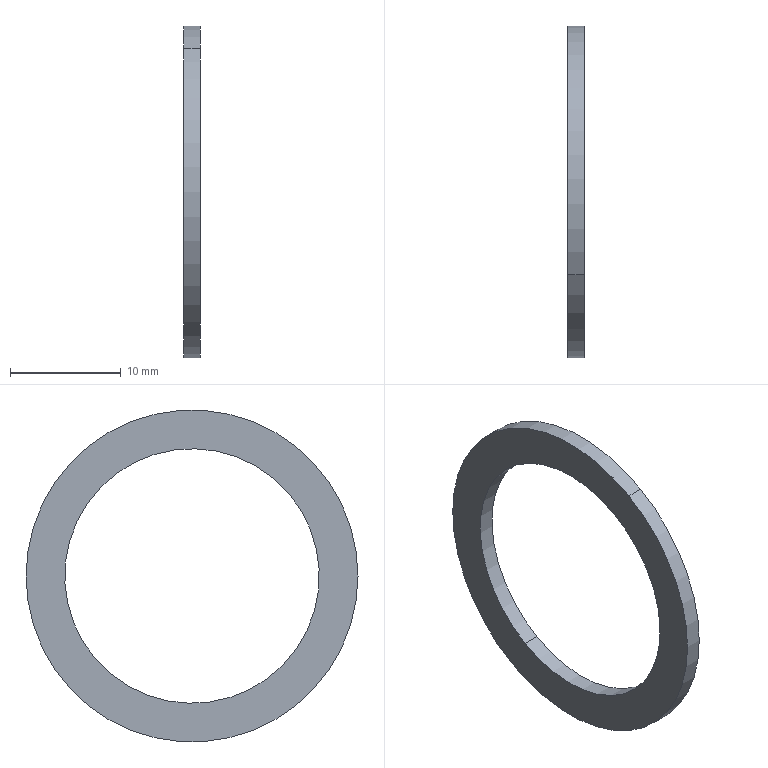Part | NX | features BREP 1 | 1 solid | 6 faces | box 1.5 x 30 x 30 mm | volume 437.074 mm3 | cylinder 4 | plane 2 | commonest cylinder face diameters 23 x2 30 x2
STEP:
#1=CARTESIAN_POINT('',(-605.855,39.831,-29.058));
#2=VERTEX_POINT('',#1);
#3=CARTESIAN_POINT('',(-605.855,51.331,-48.977));
#4=VERTEX_POINT('',#3);
#5=CARTESIAN_POINT('',(-605.855,45.581,-39.018));
#6=DIRECTION('',(-1.,0.,0.));
#7=DIRECTION('',(0.,0.5,-0.866));
#8=AXIS2_PLACEMENT_3D('',#5,#6,#7);
#9=CIRCLE('',#8,11.5);
#10=EDGE_CURVE('',#2,#4,#9,.T.);
#11=ORIENTED_EDGE('',*,*,#10,.T.);
#12=CARTESIAN_POINT('',(-604.355,51.331,-48.977));
#13=VERTEX_POINT('',#12);
#14=CARTESIAN_POINT('',(-605.855,51.331,-48.977));
#15=DIRECTION('',(-1.,0.,0.));
#16=VECTOR('',#15,1000.);
#17=LINE('',#14,#16);
#18=EDGE_CURVE('',#13,#4,#17,.T.);
#19=ORIENTED_EDGE('',*,*,#18,.F.);
#20=CARTESIAN_POINT('',(-604.355,39.831,-29.058));
#21=VERTEX_POINT('',#20);
#22=CARTESIAN_POINT('',(-604.355,45.581,-39.018));
#23=DIRECTION('',(-1.,0.,0.));
#24=DIRECTION('',(0.,0.5,-0.866));
#25=AXIS2_PLACEMENT_3D('',#22,#23,#24);
#26=CIRCLE('',#25,11.5);
#27=EDGE_CURVE('',#21,#13,#26,.T.);
#28=ORIENTED_EDGE('',*,*,#27,.F.);
#29=CARTESIAN_POINT('',(-605.855,39.831,-29.058));
#30=DIRECTION('',(-1.,0.,0.));
#31=VECTOR('',#30,1000.);
#32=LINE('',#29,#31);
#33=EDGE_CURVE('',#21,#2,#32,.T.);
#34=ORIENTED_EDGE('',*,*,#33,.T.);
#35=EDGE_LOOP('',(#11,#19,#28,#34));
#36=FACE_BOUND('',#35,.T.);
#37=CARTESIAN_POINT('',(-605.855,45.581,-39.018));
#38=DIRECTION('',(1.,0.,0.));
#39=DIRECTION('',(0.,-0.5,0.866));
#40=AXIS2_PLACEMENT_3D('',#37,#38,#39);
#41=CYLINDRICAL_SURFACE('',#40,11.5);
#42=ADVANCED_FACE('',(#36),#41,.F.);
#43=CARTESIAN_POINT('',(-605.855,53.081,-52.008));
#44=VERTEX_POINT('',#43);
#45=CARTESIAN_POINT('',(-605.855,38.081,-26.027));
#46=VERTEX_POINT('',#45);
#47=CARTESIAN_POINT('',(-605.855,45.581,-39.018));
#48=DIRECTION('',(-1.,0.,0.));
#49=DIRECTION('',(0.,0.5,-0.866));
#50=AXIS2_PLACEMENT_3D('',#47,#48,#49);
#51=CIRCLE('',#50,15.);
#52=EDGE_CURVE('',#44,#46,#51,.T.);
#53=ORIENTED_EDGE('',*,*,#52,.F.);
#54=CARTESIAN_POINT('',(-604.355,53.081,-52.008));
#55=VERTEX_POINT('',#54);
#56=CARTESIAN_POINT('',(-605.855,53.081,-52.008));
#57=DIRECTION('',(-1.,0.,0.));
#58=VECTOR('',#57,1000.);
#59=LINE('',#56,#58);
#60=EDGE_CURVE('',#55,#44,#59,.T.);
#61=ORIENTED_EDGE('',*,*,#60,.F.);
#62=CARTESIAN_POINT('',(-604.355,38.081,-26.027));
#63=VERTEX_POINT('',#62);
#64=CARTESIAN_POINT('',(-604.355,45.581,-39.018));
#65=DIRECTION('',(-1.,0.,0.));
#66=DIRECTION('',(0.,0.5,-0.866));
#67=AXIS2_PLACEMENT_3D('',#64,#65,#66);
#68=CIRCLE('',#67,15.);
#69=EDGE_CURVE('',#55,#63,#68,.T.);
#70=ORIENTED_EDGE('',*,*,#69,.T.);
#71=CARTESIAN_POINT('',(-605.855,38.081,-26.027));
#72=DIRECTION('',(-1.,0.,0.));
#73=VECTOR('',#72,1000.);
#74=LINE('',#71,#73);
#75=EDGE_CURVE('',#63,#46,#74,.T.);
#76=ORIENTED_EDGE('',*,*,#75,.T.);
#77=EDGE_LOOP('',(#53,#61,#70,#76));
#78=FACE_BOUND('',#77,.T.);
#79=CARTESIAN_POINT('',(-605.855,45.581,-39.018));
#80=DIRECTION('',(1.,0.,0.));
#81=DIRECTION('',(0.,-0.5,0.866));
#82=AXIS2_PLACEMENT_3D('',#79,#80,#81);
#83=CYLINDRICAL_SURFACE('',#82,15.);
#84=ADVANCED_FACE('',(#78),#83,.T.);
#85=CARTESIAN_POINT('',(-605.855,45.581,-39.018));
#86=DIRECTION('',(-1.,0.,0.));
#87=DIRECTION('',(0.,0.5,-0.866));
#88=AXIS2_PLACEMENT_3D('',#85,#86,#87);
#89=CIRCLE('',#88,15.);
#90=EDGE_CURVE('',#46,#44,#89,.T.);
#91=ORIENTED_EDGE('',*,*,#90,.T.);
#92=ORIENTED_EDGE('',*,*,#52,.T.);
#93=EDGE_LOOP('',(#91,#92));
#94=FACE_BOUND('',#93,.T.);
#95=ORIENTED_EDGE('',*,*,#10,.F.);
#96=CARTESIAN_POINT('',(-605.855,45.581,-39.018));
#97=DIRECTION('',(-1.,0.,0.));
#98=DIRECTION('',(0.,0.5,-0.866));
#99=AXIS2_PLACEMENT_3D('',#96,#97,#98);
#100=CIRCLE('',#99,11.5);
#101=EDGE_CURVE('',#4,#2,#100,.T.);
#102=ORIENTED_EDGE('',*,*,#101,.F.);
#103=EDGE_LOOP('',(#95,#102));
#104=FACE_BOUND('',#103,.T.);
#105=CARTESIAN_POINT('',(-605.855,45.581,-39.018));
#106=DIRECTION('',(-1.,0.,0.));
#107=DIRECTION('',(0.,0.5,-0.866));
#108=AXIS2_PLACEMENT_3D('',#105,#106,#107);
#109=PLANE('',#108);
#110=ADVANCED_FACE('',(#94,#104),#109,.T.);
#111=CARTESIAN_POINT('',(-604.355,45.581,-39.018));
#112=DIRECTION('',(-1.,0.,0.));
#113=DIRECTION('',(0.,0.5,-0.866));
#114=AXIS2_PLACEMENT_3D('',#111,#112,#113);
#115=CIRCLE('',#114,15.);
#116=EDGE_CURVE('',#63,#55,#115,.T.);
#117=ORIENTED_EDGE('',*,*,#116,.F.);
#118=ORIENTED_EDGE('',*,*,#69,.F.);
#119=EDGE_LOOP('',(#117,#118));
#120=FACE_BOUND('',#119,.T.);
#121=ORIENTED_EDGE('',*,*,#27,.T.);
#122=CARTESIAN_POINT('',(-604.355,45.581,-39.018));
#123=DIRECTION('',(-1.,0.,0.));
#124=DIRECTION('',(0.,0.5,-0.866));
#125=AXIS2_PLACEMENT_3D('',#122,#123,#124);
#126=CIRCLE('',#125,11.5);
#127=EDGE_CURVE('',#13,#21,#126,.T.);
#128=ORIENTED_EDGE('',*,*,#127,.T.);
#129=EDGE_LOOP('',(#121,#128));
#130=FACE_BOUND('',#129,.T.);
#131=CARTESIAN_POINT('',(-604.355,45.581,-39.018));
#132=DIRECTION('',(-1.,0.,0.));
#133=DIRECTION('',(0.,0.5,-0.866));
#134=AXIS2_PLACEMENT_3D('',#131,#132,#133);
#135=PLANE('',#134);
#136=ADVANCED_FACE('',(#120,#130),#135,.F.);
#137=ORIENTED_EDGE('',*,*,#60,.T.);
#138=ORIENTED_EDGE('',*,*,#90,.F.);
#139=ORIENTED_EDGE('',*,*,#75,.F.);
#140=ORIENTED_EDGE('',*,*,#116,.T.);
#141=EDGE_LOOP('',(#137,#138,#139,#140));
#142=FACE_BOUND('',#141,.T.);
#143=CARTESIAN_POINT('',(-605.855,45.581,-39.018));
#144=DIRECTION('',(1.,0.,0.));
#145=DIRECTION('',(0.,-0.5,0.866));
#146=AXIS2_PLACEMENT_3D('',#143,#144,#145);
#147=CYLINDRICAL_SURFACE('',#146,15.);
#148=ADVANCED_FACE('',(#142),#147,.T.);
#149=ORIENTED_EDGE('',*,*,#18,.T.);
#150=ORIENTED_EDGE('',*,*,#101,.T.);
#151=ORIENTED_EDGE('',*,*,#33,.F.);
#152=ORIENTED_EDGE('',*,*,#127,.F.);
#153=EDGE_LOOP('',(#149,#150,#151,#152));
#154=FACE_BOUND('',#153,.T.);
#155=CARTESIAN_POINT('',(-605.855,45.581,-39.018));
#156=DIRECTION('',(1.,0.,0.));
#157=DIRECTION('',(0.,-0.5,0.866));
#158=AXIS2_PLACEMENT_3D('',#155,#156,#157);
#159=CYLINDRICAL_SURFACE('',#158,11.5);
#160=ADVANCED_FACE('',(#154),#159,.F.);
#161=CLOSED_SHELL('',(#42,#84,#110,#136,#148,#160));
#162=MANIFOLD_SOLID_BREP('',#161);
#163=(LENGTH_UNIT()NAMED_UNIT(*)SI_UNIT(.MILLI.,.METRE.));
#164=UNCERTAINTY_MEASURE_WITH_UNIT(LENGTH_MEASURE(0.00001),#163,'','');
#165=(NAMED_UNIT(*)PLANE_ANGLE_UNIT()SI_UNIT($,.RADIAN.));
#166=(NAMED_UNIT(*)SI_UNIT($,.STERADIAN.)SOLID_ANGLE_UNIT());
#167=(GEOMETRIC_REPRESENTATION_CONTEXT(3)GLOBAL_UNCERTAINTY_ASSIGNED_CONTEXT((#164))GLOBAL_UNIT_ASSIGNED_CONTEXT((#163,#165,#166))REPRESENTATION_CONTEXT('',''));
#168=ADVANCED_BREP_SHAPE_REPRESENTATION('',(#162),#167);